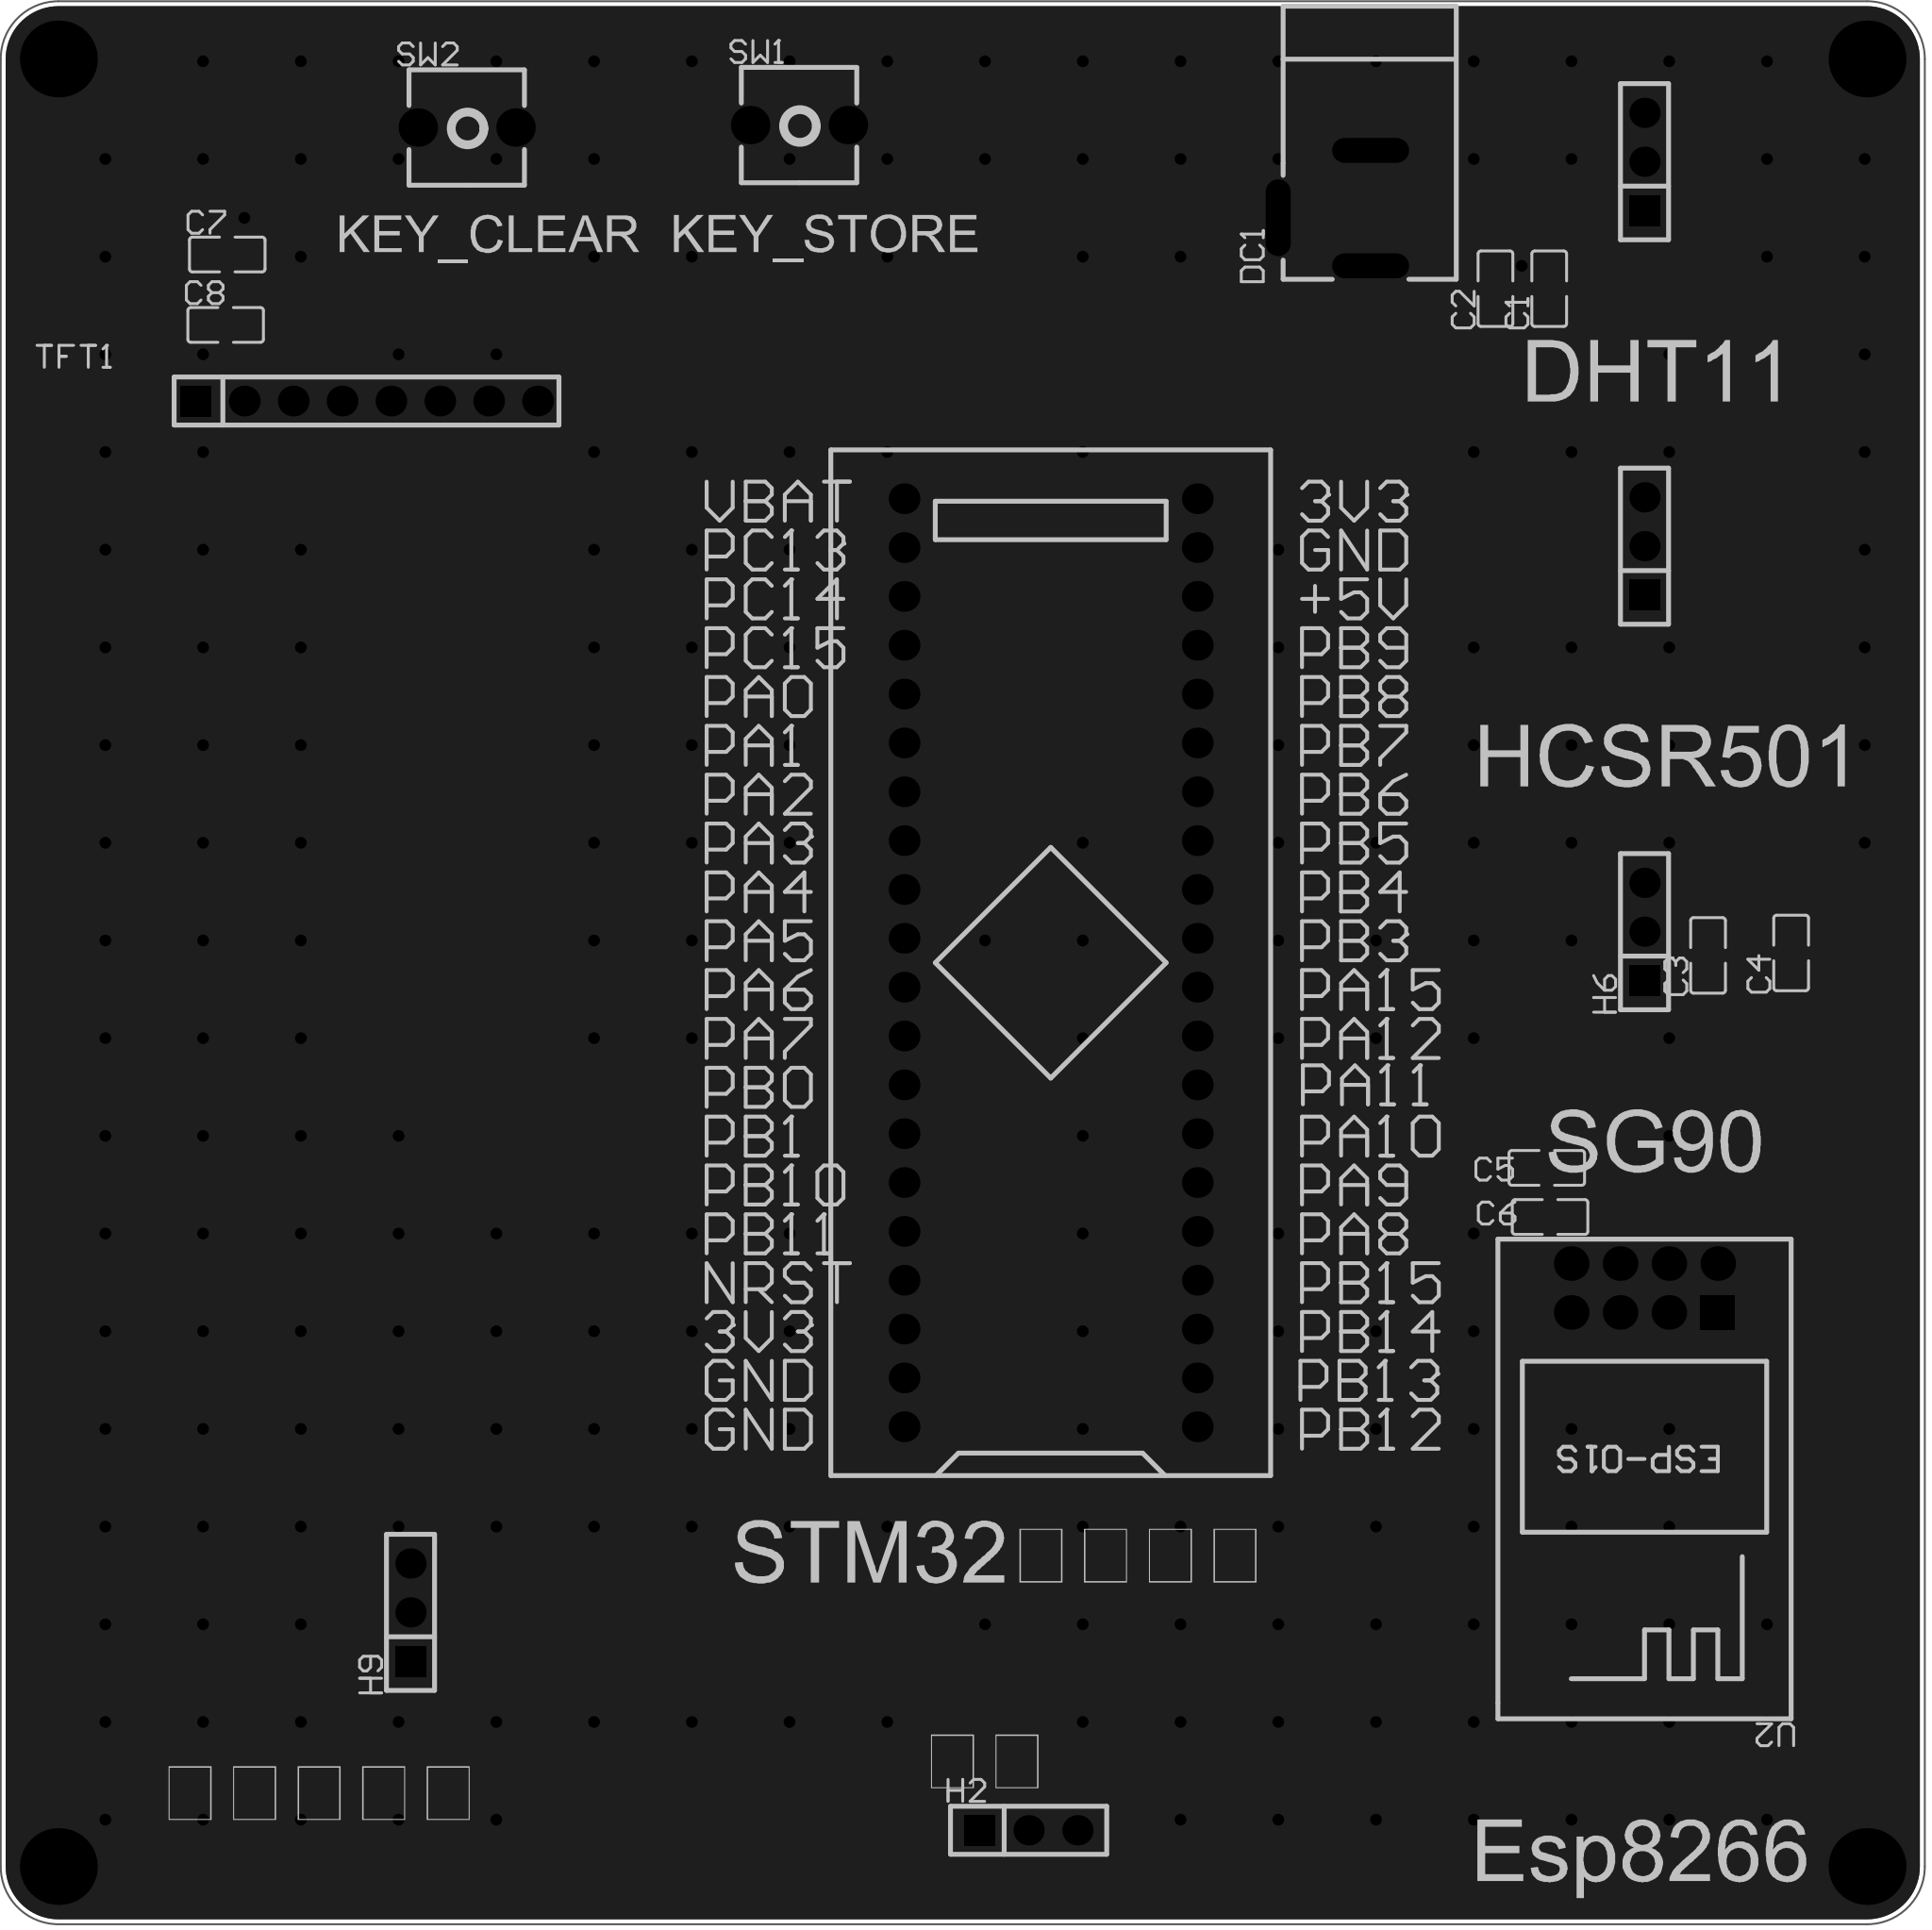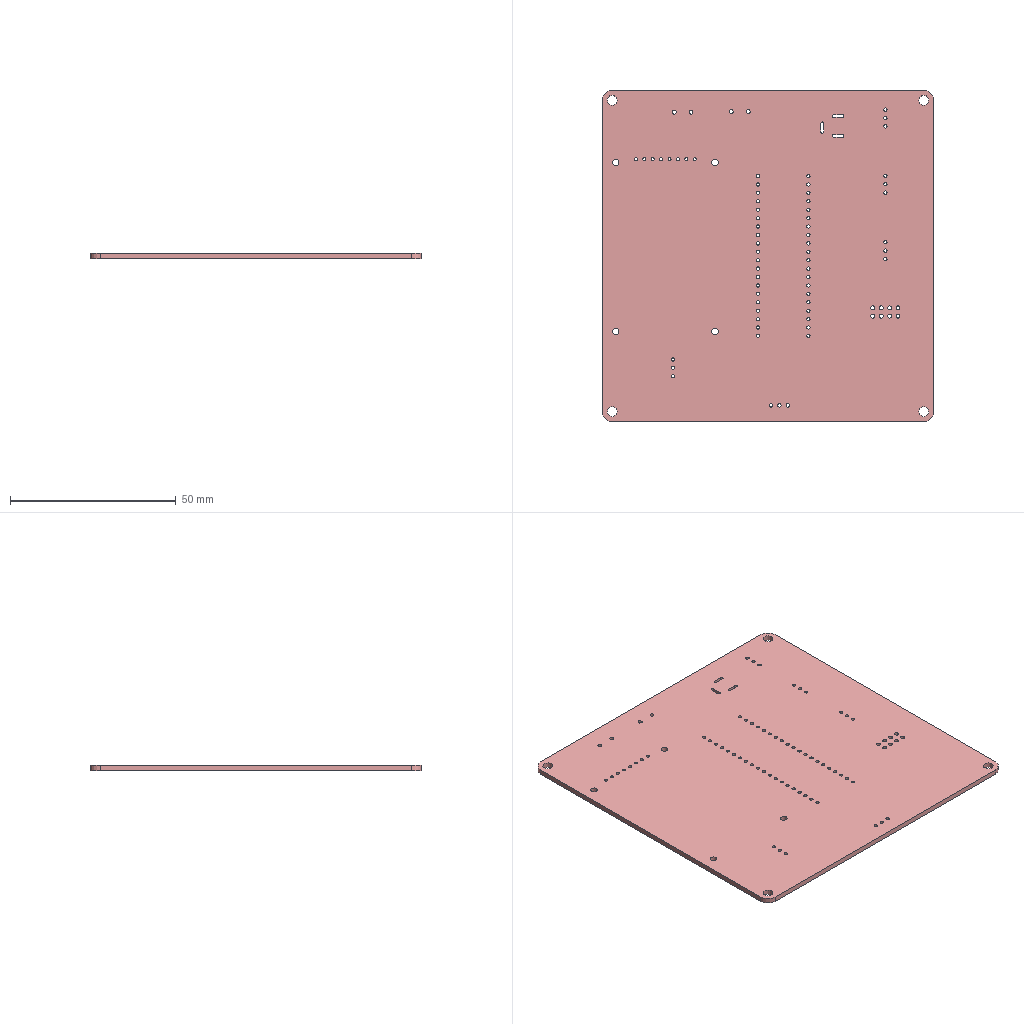Circuit board layout | Altium Designer | box 100 x 100 x 1.6 mm
Layer stack:
# Altium Designer layer stack of  (unit mm; dielectric type: 0 none, 1 core, 2 prepreg, 3 surface material)
index,name,kind,layer,copper_thickness_mm,dielectric_type,dielectric_thickness_mm,dielectric_material,dielectric_constant
0,Top Paste Mask Layer,other,,,,,,
1,Top Silkscreen Layer,other,,,,,,
2,Top Solder Mask Layer,dielectric,,,3,0.01,,3.3
3,Top Layer,copper,Top Layer,0.035,,,,
4,Dielectric1,dielectric,,,3,1.51,FR4,4.5
5,Bottom Layer,copper,Bottom Layer,0.035,,,,
6,Bottom Solder Mask Layer,dielectric,,,3,0.01,,3.3
7,Bottom Silkscreen Layer,other,,,,,,
8,Bottom Paste Mask Layer,other,,,,,,
# drill layer pairs: low layer,high layer
drill_pair,Top Layer,Bottom Layer
Part placement:
Designator,Comment,Layer,Footprint,Center-X(mm),Center-Y(mm),Rotation
U1,STM32F103C8T6-Card,TopLayer,CONN-TH_L53.3-W22.9_STM32F103C8T6-CARD,145.923,130.937,90
H1,,TopLayer,HDR-TH_3P-P2.54-V-F,176.784,152.599,90
H3,,TopLayer,HDR-TH_3P-P2.54-V-F,176.784,172.593,90
H6,,TopLayer,HDR-TH_3P-P2.54-V-F,176.784,132.553,90
DC1,,TopLayer,DC-2.0,160.147,170.18,90
H9,,TopLayer,HDR-TH_3P-P2.54-V-F,112.649,97.155,90
SW1,OMRON_B3F-6000,TopLayer,KEY-TH_2P-L6.0-W6.0-P5.00,132.842,174.498,0
TFT1,1.8 TFT 128*RGB*160,TopLayer,LCD-TH_8P-P2.54-L56.0-W34.0_1.8-TFT,110.363,160.147,0
U2,ESP-01S,TopLayer,WIFIM-TH_ESP-01S,176.784,114.023,180
C1,100uF,TopLayer,C0805,171.831,165.989,90
C2,100nF,TopLayer,C0805,169.037,165.989,90
C3,470uF,TopLayer,C0805,180.086,131.318,90
C4,100nF,TopLayer,C0805,184.404,131.445,90
C5,100uF,TopLayer,C0805,171.704,120.269,0
C6,100nF,TopLayer,C0805,171.874,117.716,0
C7,10uF,TopLayer,C0805,103.124,167.767,0
C8,100nF,TopLayer,C0805,103.04,164.104,0
SW2,OMRON_B3F-6000,TopLayer,KEY-TH_2P-L6.0-W6.0-P5.00,115.57,174.371,0
H2,,TopLayer,HDR-TH_3P-P2.54-V-F,144.774,85.823,0
Pad and via stacks:
# Altium Designer via and pad stacks of  (unit mm). Each distinct definition once, with the count of objects using it.
# via: kind,start_layer,end_layer,hole_mm,diameter_mm,mode(0 simple;1 top-mid-bottom;2 full stack),diameter_per_layer,count,example_net
# pad: kind,layer,hole_mm,hole_type(0 round;1 square;2 slot),plating,top_size,top_shape(1 round;2 rect;3 octagon;9 rounded rect),mid_size,bottom_size,mode,footprint,size_per_layer,count,example
pad,Multi-Layer,3,0,plated,4x4,1,4x4,4x4,0,,,4,1
pad,Multi-Layer,1,0,plated,1.6x1.6,1,1.6x1.6,1.6x1.6,0,CONN-TH_L53.3-W22.9_STM32F103C8T6-CARD,,40,U1.1
pad,Multi-Layer,1.02,0,plated,1.575x1.575,1,1.575x1.575,1.575x1.575,0,HDR-TH_3P-P2.54-V-F,,10,H1.3
pad,Multi-Layer,1.02,0,plated,1.575x1.575,2,1.575x1.575,1.575x1.575,0,HDR-TH_3P-P2.54-V-F,,5,H1.1
pad,Multi-Layer,0.8001,2,plated,4x1.3,1,4x1.3,4x1.3,0,DC-2.0,,3,DC1.2
pad,Multi-Layer,1.2,0,plated,2x2,1,2x2,2x2,0,KEY-TH_2P-L6.0-W6.0-P5.00,,4,SW1.2
pad,Multi-Layer,0.9144,0,plated,1.6x1.6,2,1.6x1.6,1.6x1.6,0,LCD-TH_8P-P2.54-L56.0-W34.0_1.8-TFT,,1,TFT1.1
pad,Multi-Layer,0.9144,0,plated,1.6x1.6,1,1.6x1.6,1.6x1.6,0,LCD-TH_8P-P2.54-L56.0-W34.0_1.8-TFT,,7,TFT1.2
pad,Multi-Layer,1.2,0,plated,1.8x1.8,2,1.8x1.8,1.8x1.8,0,WIFIM-TH_ESP-01S,,1,U2.1
pad,Multi-Layer,1.2,0,plated,1.8x1.8,1,1.8x1.8,1.8x1.8,0,WIFIM-TH_ESP-01S,,7,U2.2
pad,Top Layer,0,0,plated,1.41x1.35,2,1.41x1.35,1.41x1.35,0,C0805,,16,C1.2
via,Top Layer,Bottom Layer,0.3048,0.61,0,,225,+5V
Copper pours:
name,layer,net,type(0 solid;1 hatched;2 none)
Bottom Layer-GND,Bottom Layer,GND,0
Top Layer-GND,Top Layer,GND,0
Design rules, without the lines most boards share:
# Altium Designer design rules of  (exported by Altium Designer, unit mm)
# columns: name | kind | enabled | priority | scope1 | scope2 | descriptor | typed fields (field=value)
Copper_copperRegion_copperThickness1oz | 0 | disabled | 4 | All | All | Clearance Constraint (Gap=5.984mil) (Disabled)(All),(All) | gap=0.152
Copper_copperRegion_copperThickness1oz_1 | 63 | disabled | 4 | All | All | Board Clearance Constraint (Gap=0mil) (Disabled)(All) |
Copper_copperRegion_Copper_copperRegion | 0 | disabled | 5 | All | All | Clearance Constraint (Gap=5.984mil) (Disabled)(All),(All) | gap=0.152
Copper_copperRegion_Copper_copperRegion_1 | 63 | disabled | 5 | All | All | Board Clearance Constraint (Gap=0mil) (Disabled)(All) |
copperThickness1oz | 0 | enabled | 6 | All | All | Clearance Constraint (Gap=5.984mil) (All),(All) | gap=0.152
copperThickness1oz_1 | 63 | enabled | 6 | All | All | Board Clearance Constraint (Gap=0mil) (All) |
copperRegion_copperThickness1oz | 20 | disabled | 1 | All | All | Polygon Connect Rule(Relief Connect )(Conductor Width=10mil) (Relief Angle=90 Angle) (Entries=4) (Air Gap Width=10mil) (Disabled)(All),(All) | connect_style(0=relief,1=direct,2=none)=0 relief_conductor_width=0.254 relief_entries=4
copperRegion_Copper_copperRegion | 20 | disabled | 2 | All | All | Polygon Connect Rule(Relief Connect )(Conductor Width=10mil) (Relief Angle=90 Angle) (Entries=4) (Air Gap Width=10mil) (Disabled)(All),(All) | connect_style(0=relief,1=direct,2=none)=0 relief_conductor_width=0.254 relief_entries=4
copperRegion | 20 | enabled | 3 | All | All | Polygon Connect Rule(Relief Connect )(Conductor Width=10mil) (Relief Angle=90 Angle) (Entries=4) (Air Gap Width=10mil) (All),(All) | connect_style(0=relief,1=direct,2=none)=0 relief_conductor_width=0.254 relief_entries=4